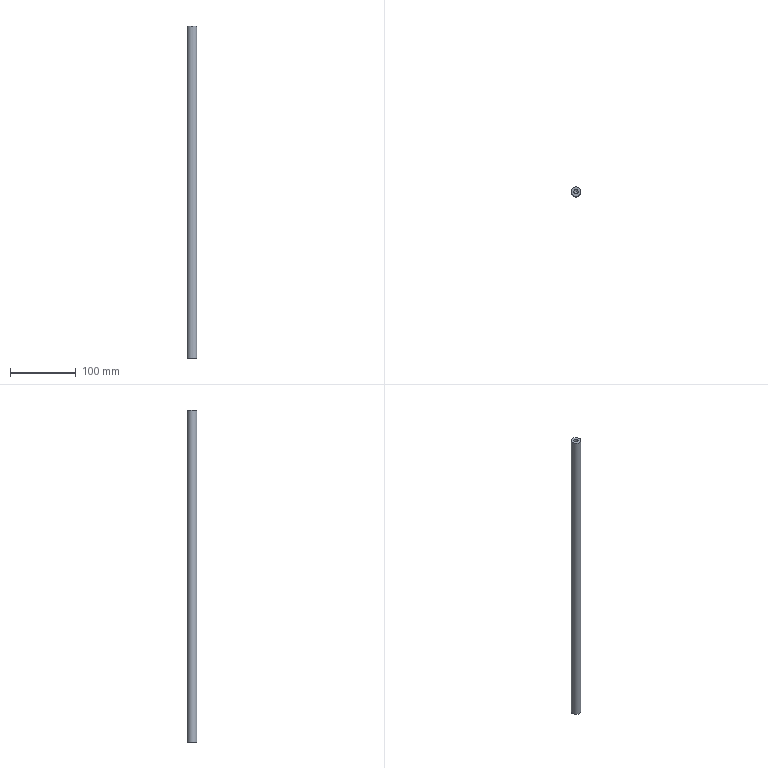Part | STEP file | axe506 | 1 solid | 7 faces | box 15 x 15 x 506 mm | volume 87993 mm3 | spline 4 | plane 2 | cylinder 1 | commonest cylinder face diameters 15 x1
STEP:
#1=CARTESIAN_POINT('',(0.,0.,0.));
#2=DIRECTION('',(0.,0.,1.));
#3=DIRECTION('',(1.,0.,0.));
#4=AXIS2_PLACEMENT_3D('',#1,#2,#3);
#5=CARTESIAN_POINT('',(3.324,0.,20.));
#6=VERTEX_POINT('',#5);
#7=CARTESIAN_POINT('',(-3.324,0.,20.));
#8=VERTEX_POINT('',#7);
#9=CARTESIAN_POINT('',(0.,0.,20.));
#10=DIRECTION('',(0.,0.,-1.));
#11=DIRECTION('',(-1.,0.,0.));
#12=AXIS2_PLACEMENT_3D('',#9,#10,#11);
#13=CIRCLE('',#12,3.324);
#14=CARTESIAN_POINT('',(3.324,0.,20.));
#15=CARTESIAN_POINT('',(3.324,-3.324,20.));
#16=CARTESIAN_POINT('',(0.,-3.324,20.));
#17=CARTESIAN_POINT('',(-3.324,-3.324,20.));
#18=CARTESIAN_POINT('',(-3.324,0.,20.));
#19=CARTESIAN_POINT('',(-3.324,3.324,20.));
#20=CARTESIAN_POINT('',(0.,3.324,20.));
#21=CARTESIAN_POINT('',(3.324,3.324,20.));
#22=CARTESIAN_POINT('',(3.324,0.,20.));
#23=CARTESIAN_POINT('',(0.,0.,21.997));
#24=CARTESIAN_POINT('',(0.,0.,21.997));
#25=CARTESIAN_POINT('',(0.,0.,21.997));
#26=CARTESIAN_POINT('',(0.,0.,21.997));
#27=CARTESIAN_POINT('',(0.,0.,21.997));
#28=CARTESIAN_POINT('',(0.,0.,21.997));
#29=CARTESIAN_POINT('',(0.,0.,21.997));
#30=CARTESIAN_POINT('',(0.,0.,21.997));
#31=CARTESIAN_POINT('',(0.,0.,21.997));
#32=(BOUNDED_SURFACE()B_SPLINE_SURFACE(1,2,((#14,#15,#16,#17,#18,#19,#20,#21,#22),(#23,#24,#25,#26,#27,#28,#29,#30,#31)),.UNSPECIFIED.,.F.,.T.,.F.)B_SPLINE_SURFACE_WITH_KNOTS((2,2),(1,2,2,2,2,2,1),(-1.167,1.167),(-2.61,0.,2.61,5.221,7.831,10.441,13.051),.UNSPECIFIED.)GEOMETRIC_REPRESENTATION_ITEM()RATIONAL_B_SPLINE_SURFACE(((1.,0.7071,1.,0.7071,1.,0.7071,1.,0.7071,1.),(1.,0.7071,1.,0.7071,1.,0.7071,1.,0.7071,1.)))REPRESENTATION_ITEM('')SURFACE());
#33=CARTESIAN_POINT('',(-1.167,-5.221));
#34=CARTESIAN_POINT('',(-1.167,-5.045));
#35=CARTESIAN_POINT('',(-1.167,-4.714));
#36=CARTESIAN_POINT('',(-1.167,-4.252));
#37=CARTESIAN_POINT('',(-1.167,-3.804));
#38=CARTESIAN_POINT('',(-1.167,-3.35));
#39=CARTESIAN_POINT('',(-1.167,-2.876));
#40=CARTESIAN_POINT('',(-1.167,-2.344));
#41=CARTESIAN_POINT('',(-1.167,-1.87));
#42=CARTESIAN_POINT('',(-1.167,-1.417));
#43=CARTESIAN_POINT('',(-1.167,-0.968));
#44=CARTESIAN_POINT('',(-1.167,-0.5094));
#45=CARTESIAN_POINT('',(-1.167,0.));
#46=CARTESIAN_POINT('',(-1.167,0.5094));
#47=CARTESIAN_POINT('',(-1.167,0.968));
#48=CARTESIAN_POINT('',(-1.167,1.417));
#49=CARTESIAN_POINT('',(-1.167,1.87));
#50=CARTESIAN_POINT('',(-1.167,2.344));
#51=CARTESIAN_POINT('',(-1.167,2.876));
#52=CARTESIAN_POINT('',(-1.167,3.35));
#53=CARTESIAN_POINT('',(-1.167,3.804));
#54=CARTESIAN_POINT('',(-1.167,4.252));
#55=CARTESIAN_POINT('',(-1.167,4.714));
#56=CARTESIAN_POINT('',(-1.167,5.045));
#57=CARTESIAN_POINT('',(-1.167,5.221));
#58=B_SPLINE_CURVE_WITH_KNOTS('',3,(#33,#34,#35,#36,#37,#38,#39,#40,#41,#42,#43,#44,#45,#46,#47,#48,#49,#50,#51,#52,#53,#54,#55,#56,#57),.UNSPECIFIED.,.F.,.F.,(4,1,1,1,1,1,1,1,1,1,1,1,1,1,1,1,1,1,1,1,1,1,4),(0.,0.2856,0.5712,0.8568,1.142,1.428,1.714,1.999,2.285,2.57,2.856,3.142,3.427,3.713,3.998,4.284,4.57,4.855,5.141,5.426,5.712,5.998,6.283),.QUASI_UNIFORM_KNOTS.);
#59=(GEOMETRIC_REPRESENTATION_CONTEXT(2)PARAMETRIC_REPRESENTATION_CONTEXT()REPRESENTATION_CONTEXT('',''));
#60=DEFINITIONAL_REPRESENTATION('',(#58),#59);
#61=PCURVE('',#32,#60);
#62=CARTESIAN_POINT('',(3.324,0.,0.));
#63=CARTESIAN_POINT('',(3.324,-3.324,0.));
#64=CARTESIAN_POINT('',(0.,-3.324,0.));
#65=CARTESIAN_POINT('',(-3.324,-3.324,0.));
#66=CARTESIAN_POINT('',(-3.324,0.,0.));
#67=CARTESIAN_POINT('',(-3.324,3.324,0.));
#68=CARTESIAN_POINT('',(0.,3.324,0.));
#69=CARTESIAN_POINT('',(3.324,3.324,0.));
#70=CARTESIAN_POINT('',(3.324,0.,0.));
#71=CARTESIAN_POINT('',(3.324,0.,20.));
#72=CARTESIAN_POINT('',(3.324,-3.324,20.));
#73=CARTESIAN_POINT('',(0.,-3.324,20.));
#74=CARTESIAN_POINT('',(-3.324,-3.324,20.));
#75=CARTESIAN_POINT('',(-3.324,0.,20.));
#76=CARTESIAN_POINT('',(-3.324,3.324,20.));
#77=CARTESIAN_POINT('',(0.,3.324,20.));
#78=CARTESIAN_POINT('',(3.324,3.324,20.));
#79=CARTESIAN_POINT('',(3.324,0.,20.));
#80=(BOUNDED_SURFACE()B_SPLINE_SURFACE(1,2,((#62,#63,#64,#65,#66,#67,#68,#69,#70),(#71,#72,#73,#74,#75,#76,#77,#78,#79)),.UNSPECIFIED.,.F.,.T.,.F.)B_SPLINE_SURFACE_WITH_KNOTS((2,2),(1,2,2,2,2,2,1),(-3.009,3.009),(-5.221,0.,5.221,10.441,15.662,20.882,26.103),.UNSPECIFIED.)GEOMETRIC_REPRESENTATION_ITEM()RATIONAL_B_SPLINE_SURFACE(((1.,0.7071,1.,0.7071,1.,0.7071,1.,0.7071,1.),(1.,0.7071,1.,0.7071,1.,0.7071,1.,0.7071,1.)))REPRESENTATION_ITEM('')SURFACE());
#81=CARTESIAN_POINT('',(3.009,20.882));
#82=CARTESIAN_POINT('',(3.009,21.058));
#83=CARTESIAN_POINT('',(3.009,21.399));
#84=CARTESIAN_POINT('',(3.009,21.887));
#85=CARTESIAN_POINT('',(3.009,22.357));
#86=CARTESIAN_POINT('',(3.009,22.816));
#87=CARTESIAN_POINT('',(3.009,23.268));
#88=CARTESIAN_POINT('',(3.009,23.717));
#89=CARTESIAN_POINT('',(3.009,24.169));
#90=CARTESIAN_POINT('',(3.009,24.627));
#91=CARTESIAN_POINT('',(3.009,25.098));
#92=CARTESIAN_POINT('',(3.009,25.585));
#93=CARTESIAN_POINT('',(3.009,26.103));
#94=CARTESIAN_POINT('',(3.009,26.621));
#95=CARTESIAN_POINT('',(3.009,27.107));
#96=CARTESIAN_POINT('',(3.009,27.578));
#97=CARTESIAN_POINT('',(3.009,28.037));
#98=CARTESIAN_POINT('',(3.009,28.488));
#99=CARTESIAN_POINT('',(3.009,28.938));
#100=CARTESIAN_POINT('',(3.009,29.389));
#101=CARTESIAN_POINT('',(3.009,29.848));
#102=CARTESIAN_POINT('',(3.009,30.319));
#103=CARTESIAN_POINT('',(3.009,30.806));
#104=CARTESIAN_POINT('',(3.009,31.148));
#105=CARTESIAN_POINT('',(3.009,31.323));
#106=B_SPLINE_CURVE_WITH_KNOTS('',3,(#81,#82,#83,#84,#85,#86,#87,#88,#89,#90,#91,#92,#93,#94,#95,#96,#97,#98,#99,#100,#101,#102,#103,#104,#105),.UNSPECIFIED.,.F.,.F.,(4,1,1,1,1,1,1,1,1,1,1,1,1,1,1,1,1,1,1,1,1,1,4),(3.142,3.284,3.427,3.57,3.713,3.856,3.998,4.141,4.284,4.427,4.57,4.712,4.855,4.998,5.141,5.284,5.426,5.569,5.712,5.855,5.998,6.14,6.283),.QUASI_UNIFORM_KNOTS.);
#107=(GEOMETRIC_REPRESENTATION_CONTEXT(2)PARAMETRIC_REPRESENTATION_CONTEXT()REPRESENTATION_CONTEXT('',''));
#108=DEFINITIONAL_REPRESENTATION('',(#106),#107);
#109=PCURVE('',#80,#108);
#110=SURFACE_CURVE('',#13,(#61,#109),.PCURVE_S1.);
#111=EDGE_CURVE('',#6,#8,#110,.T.);
#112=ORIENTED_EDGE('',*,*,#111,.F.);
#113=CARTESIAN_POINT('',(0.,0.,21.997));
#114=VERTEX_POINT('',#113);
#115=CARTESIAN_POINT('',(3.324,0.,20.));
#116=CARTESIAN_POINT('',(0.,0.,21.997));
#117=B_SPLINE_CURVE_WITH_KNOTS('',1,(#115,#116),.UNSPECIFIED.,.F.,.F.,(2,2),(-1.167,1.167),.PIECEWISE_BEZIER_KNOTS.);
#118=CARTESIAN_POINT('',(0.,0.));
#119=DIRECTION('',(1.,0.));
#120=VECTOR('',#119,1.);
#121=LINE('',#118,#120);
#122=(GEOMETRIC_REPRESENTATION_CONTEXT(2)PARAMETRIC_REPRESENTATION_CONTEXT()REPRESENTATION_CONTEXT('',''));
#123=DEFINITIONAL_REPRESENTATION('',(#121),#122);
#124=PCURVE('',#32,#123);
#125=CARTESIAN_POINT('',(0.,10.441));
#126=DIRECTION('',(1.,0.));
#127=VECTOR('',#126,1.);
#128=LINE('',#125,#127);
#129=(GEOMETRIC_REPRESENTATION_CONTEXT(2)PARAMETRIC_REPRESENTATION_CONTEXT()REPRESENTATION_CONTEXT('',''));
#130=DEFINITIONAL_REPRESENTATION('',(#128),#129);
#131=PCURVE('',#32,#130);
#132=SEAM_CURVE('',#117,(#124,#131),.PCURVE_S1.);
#133=EDGE_CURVE('',#6,#114,#132,.T.);
#134=ORIENTED_EDGE('',*,*,#133,.T.);
#135=ORIENTED_EDGE('',*,*,#133,.F.);
#136=CARTESIAN_POINT('',(0.,0.,20.));
#137=DIRECTION('',(0.,0.,-1.));
#138=DIRECTION('',(-1.,0.,0.));
#139=AXIS2_PLACEMENT_3D('',#136,#137,#138);
#140=CIRCLE('',#139,3.324);
#141=CARTESIAN_POINT('',(-1.167,5.221));
#142=CARTESIAN_POINT('',(-1.167,5.396));
#143=CARTESIAN_POINT('',(-1.167,5.727));
#144=CARTESIAN_POINT('',(-1.167,6.189));
#145=CARTESIAN_POINT('',(-1.167,6.637));
#146=CARTESIAN_POINT('',(-1.167,7.091));
#147=CARTESIAN_POINT('',(-1.167,7.565));
#148=CARTESIAN_POINT('',(-1.167,8.097));
#149=CARTESIAN_POINT('',(-1.167,8.571));
#150=CARTESIAN_POINT('',(-1.167,9.024));
#151=CARTESIAN_POINT('',(-1.167,9.473));
#152=CARTESIAN_POINT('',(-1.167,9.932));
#153=CARTESIAN_POINT('',(-1.167,10.441));
#154=CARTESIAN_POINT('',(-1.167,10.95));
#155=CARTESIAN_POINT('',(-1.167,11.409));
#156=CARTESIAN_POINT('',(-1.167,11.858));
#157=CARTESIAN_POINT('',(-1.167,12.311));
#158=CARTESIAN_POINT('',(-1.167,12.785));
#159=CARTESIAN_POINT('',(-1.167,13.318));
#160=CARTESIAN_POINT('',(-1.167,13.791));
#161=CARTESIAN_POINT('',(-1.167,14.245));
#162=CARTESIAN_POINT('',(-1.167,14.693));
#163=CARTESIAN_POINT('',(-1.167,15.155));
#164=CARTESIAN_POINT('',(-1.167,15.486));
#165=CARTESIAN_POINT('',(-1.167,15.662));
#166=B_SPLINE_CURVE_WITH_KNOTS('',3,(#141,#142,#143,#144,#145,#146,#147,#148,#149,#150,#151,#152,#153,#154,#155,#156,#157,#158,#159,#160,#161,#162,#163,#164,#165),.UNSPECIFIED.,.F.,.F.,(4,1,1,1,1,1,1,1,1,1,1,1,1,1,1,1,1,1,1,1,1,1,4),(0.,0.2856,0.5712,0.8568,1.142,1.428,1.714,1.999,2.285,2.57,2.856,3.142,3.427,3.713,3.998,4.284,4.57,4.855,5.141,5.426,5.712,5.998,6.283),.QUASI_UNIFORM_KNOTS.);
#167=(GEOMETRIC_REPRESENTATION_CONTEXT(2)PARAMETRIC_REPRESENTATION_CONTEXT()REPRESENTATION_CONTEXT('',''));
#168=DEFINITIONAL_REPRESENTATION('',(#166),#167);
#169=PCURVE('',#32,#168);
#170=CARTESIAN_POINT('',(3.009,10.441));
#171=CARTESIAN_POINT('',(3.009,10.617));
#172=CARTESIAN_POINT('',(3.009,10.958));
#173=CARTESIAN_POINT('',(3.009,11.446));
#174=CARTESIAN_POINT('',(3.009,11.916));
#175=CARTESIAN_POINT('',(3.009,12.375));
#176=CARTESIAN_POINT('',(3.009,12.827));
#177=CARTESIAN_POINT('',(3.009,13.276));
#178=CARTESIAN_POINT('',(3.009,13.728));
#179=CARTESIAN_POINT('',(3.009,14.186));
#180=CARTESIAN_POINT('',(3.009,14.657));
#181=CARTESIAN_POINT('',(3.009,15.143));
#182=CARTESIAN_POINT('',(3.009,15.662));
#183=CARTESIAN_POINT('',(3.009,16.18));
#184=CARTESIAN_POINT('',(3.009,16.666));
#185=CARTESIAN_POINT('',(3.009,17.137));
#186=CARTESIAN_POINT('',(3.009,17.596));
#187=CARTESIAN_POINT('',(3.009,18.047));
#188=CARTESIAN_POINT('',(3.009,18.497));
#189=CARTESIAN_POINT('',(3.009,18.948));
#190=CARTESIAN_POINT('',(3.009,19.407));
#191=CARTESIAN_POINT('',(3.009,19.877));
#192=CARTESIAN_POINT('',(3.009,20.365));
#193=CARTESIAN_POINT('',(3.009,20.707));
#194=CARTESIAN_POINT('',(3.009,20.882));
#195=B_SPLINE_CURVE_WITH_KNOTS('',3,(#170,#171,#172,#173,#174,#175,#176,#177,#178,#179,#180,#181,#182,#183,#184,#185,#186,#187,#188,#189,#190,#191,#192,#193,#194),.UNSPECIFIED.,.F.,.F.,(4,1,1,1,1,1,1,1,1,1,1,1,1,1,1,1,1,1,1,1,1,1,4),(0.,0.1428,0.2856,0.4284,0.5712,0.714,0.8568,0.9996,1.142,1.285,1.428,1.571,1.714,1.856,1.999,2.142,2.285,2.428,2.57,2.713,2.856,2.999,3.142),.QUASI_UNIFORM_KNOTS.);
#196=(GEOMETRIC_REPRESENTATION_CONTEXT(2)PARAMETRIC_REPRESENTATION_CONTEXT()REPRESENTATION_CONTEXT('',''));
#197=DEFINITIONAL_REPRESENTATION('',(#195),#196);
#198=PCURVE('',#80,#197);
#199=SURFACE_CURVE('',#140,(#169,#198),.PCURVE_S1.);
#200=EDGE_CURVE('',#8,#6,#199,.T.);
#201=ORIENTED_EDGE('',*,*,#200,.F.);
#202=EDGE_LOOP('',(#112,#134,#135,#201));
#203=FACE_BOUND('',#202,.F.);
#204=ADVANCED_FACE('',(#203),#32,.F.);
#205=CARTESIAN_POINT('',(-3.324,0.,0.));
#206=VERTEX_POINT('',#205);
#207=CARTESIAN_POINT('',(0.,0.,0.));
#208=DIRECTION('',(0.,0.,1.));
#209=DIRECTION('',(-1.,0.,0.));
#210=AXIS2_PLACEMENT_3D('',#207,#208,#209);
#211=CIRCLE('',#210,3.324);
#212=CARTESIAN_POINT('',(-3.009,31.323));
#213=CARTESIAN_POINT('',(-3.009,30.973));
#214=CARTESIAN_POINT('',(-3.009,30.31));
#215=CARTESIAN_POINT('',(-3.009,29.386));
#216=CARTESIAN_POINT('',(-3.009,28.49));
#217=CARTESIAN_POINT('',(-3.009,27.583));
#218=CARTESIAN_POINT('',(-3.009,26.635));
#219=CARTESIAN_POINT('',(-3.009,25.57));
#220=CARTESIAN_POINT('',(-3.009,24.622));
#221=CARTESIAN_POINT('',(-3.009,23.716));
#222=CARTESIAN_POINT('',(-3.009,22.818));
#223=CARTESIAN_POINT('',(-3.009,21.901));
#224=CARTESIAN_POINT('',(-3.009,20.882));
#225=CARTESIAN_POINT('',(-3.009,19.863));
#226=CARTESIAN_POINT('',(-3.009,18.946));
#227=CARTESIAN_POINT('',(-3.009,18.048));
#228=CARTESIAN_POINT('',(-3.009,17.142));
#229=CARTESIAN_POINT('',(-3.009,16.194));
#230=CARTESIAN_POINT('',(-3.009,15.129));
#231=CARTESIAN_POINT('',(-3.009,14.181));
#232=CARTESIAN_POINT('',(-3.009,13.275));
#233=CARTESIAN_POINT('',(-3.009,12.378));
#234=CARTESIAN_POINT('',(-3.009,11.455));
#235=CARTESIAN_POINT('',(-3.009,10.792));
#236=CARTESIAN_POINT('',(-3.009,10.441));
#237=B_SPLINE_CURVE_WITH_KNOTS('',3,(#212,#213,#214,#215,#216,#217,#218,#219,#220,#221,#222,#223,#224,#225,#226,#227,#228,#229,#230,#231,#232,#233,#234,#235,#236),.UNSPECIFIED.,.F.,.F.,(4,1,1,1,1,1,1,1,1,1,1,1,1,1,1,1,1,1,1,1,1,1,4),(0.,0.2856,0.5712,0.8568,1.142,1.428,1.714,1.999,2.285,2.57,2.856,3.142,3.427,3.713,3.998,4.284,4.57,4.855,5.141,5.426,5.712,5.998,6.283),.QUASI_UNIFORM_KNOTS.);
#238=(GEOMETRIC_REPRESENTATION_CONTEXT(2)PARAMETRIC_REPRESENTATION_CONTEXT()REPRESENTATION_CONTEXT('',''));
#239=DEFINITIONAL_REPRESENTATION('',(#237),#238);
#240=PCURVE('',#80,#239);
#241=CARTESIAN_POINT('',(0.,0.,0.));
#242=DIRECTION('',(0.,0.,-1.));
#243=DIRECTION('',(-1.,0.,0.));
#244=AXIS2_PLACEMENT_3D('',#241,#242,#243);
#245=PLANE('',#244);
#246=CARTESIAN_POINT('',(3.324,0.));
#247=CARTESIAN_POINT('',(3.324,-5.756));
#248=CARTESIAN_POINT('',(-1.662,-2.878));
#249=CARTESIAN_POINT('',(-6.647,0.));
#250=CARTESIAN_POINT('',(-1.662,2.878));
#251=CARTESIAN_POINT('',(3.324,5.756));
#252=CARTESIAN_POINT('',(3.324,0.));
#253=(BOUNDED_CURVE()B_SPLINE_CURVE(2,(#246,#247,#248,#249,#250,#251,#252),.UNSPECIFIED.,.T.,.F.)B_SPLINE_CURVE_WITH_KNOTS((1,2,2,2,2,1),(-2.094,0.,2.094,4.189,6.283,8.378),.UNSPECIFIED.)CURVE()GEOMETRIC_REPRESENTATION_ITEM()RATIONAL_B_SPLINE_CURVE((1.,0.5,1.,0.5,1.,0.5,1.))REPRESENTATION_ITEM(''));
#254=(GEOMETRIC_REPRESENTATION_CONTEXT(2)PARAMETRIC_REPRESENTATION_CONTEXT()REPRESENTATION_CONTEXT('',''));
#255=DEFINITIONAL_REPRESENTATION('',(#253),#254);
#256=PCURVE('',#245,#255);
#257=SURFACE_CURVE('',#211,(#240,#256),.PCURVE_S1.);
#258=EDGE_CURVE('',#206,#206,#257,.T.);
#259=ORIENTED_EDGE('',*,*,#258,.T.);
#260=CARTESIAN_POINT('',(-3.324,0.,0.));
#261=CARTESIAN_POINT('',(-3.324,0.,20.));
#262=B_SPLINE_CURVE_WITH_KNOTS('',1,(#260,#261),.UNSPECIFIED.,.F.,.F.,(2,2),(-3.009,3.009),.PIECEWISE_BEZIER_KNOTS.);
#263=CARTESIAN_POINT('',(0.,10.441));
#264=DIRECTION('',(1.,0.));
#265=VECTOR('',#264,1.);
#266=LINE('',#263,#265);
#267=(GEOMETRIC_REPRESENTATION_CONTEXT(2)PARAMETRIC_REPRESENTATION_CONTEXT()REPRESENTATION_CONTEXT('',''));
#268=DEFINITIONAL_REPRESENTATION('',(#266),#267);
#269=PCURVE('',#80,#268);
#270=CARTESIAN_POINT('',(0.,31.323));
#271=DIRECTION('',(1.,0.));
#272=VECTOR('',#271,1.);
#273=LINE('',#270,#272);
#274=(GEOMETRIC_REPRESENTATION_CONTEXT(2)PARAMETRIC_REPRESENTATION_CONTEXT()REPRESENTATION_CONTEXT('',''));
#275=DEFINITIONAL_REPRESENTATION('',(#273),#274);
#276=PCURVE('',#80,#275);
#277=SEAM_CURVE('',#262,(#269,#276),.PCURVE_S1.);
#278=EDGE_CURVE('',#206,#8,#277,.T.);
#279=ORIENTED_EDGE('',*,*,#278,.T.);
#280=ORIENTED_EDGE('',*,*,#200,.T.);
#281=ORIENTED_EDGE('',*,*,#111,.T.);
#282=ORIENTED_EDGE('',*,*,#278,.F.);
#283=EDGE_LOOP('',(#259,#279,#280,#281,#282));
#284=FACE_BOUND('',#283,.F.);
#285=ADVANCED_FACE('',(#284),#80,.F.);
#286=CARTESIAN_POINT('',(-3.324,0.,486.));
#287=VERTEX_POINT('',#286);
#288=CARTESIAN_POINT('',(3.324,0.,486.));
#289=VERTEX_POINT('',#288);
#290=CARTESIAN_POINT('',(0.,0.,486.));
#291=DIRECTION('',(0.,0.,1.));
#292=DIRECTION('',(1.,0.,0.));
#293=AXIS2_PLACEMENT_3D('',#290,#291,#292);
#294=CIRCLE('',#293,3.324);
#295=CARTESIAN_POINT('',(-3.324,0.,486.));
#296=CARTESIAN_POINT('',(-3.324,-3.324,486.));
#297=CARTESIAN_POINT('',(0.,-3.324,486.));
#298=CARTESIAN_POINT('',(3.324,-3.324,486.));
#299=CARTESIAN_POINT('',(3.324,0.,486.));
#300=CARTESIAN_POINT('',(3.324,3.324,486.));
#301=CARTESIAN_POINT('',(0.,3.324,486.));
#302=CARTESIAN_POINT('',(-3.324,3.324,486.));
#303=CARTESIAN_POINT('',(-3.324,0.,486.));
#304=CARTESIAN_POINT('',(0.,0.,484.003));
#305=CARTESIAN_POINT('',(0.,0.,484.003));
#306=CARTESIAN_POINT('',(0.,0.,484.003));
#307=CARTESIAN_POINT('',(0.,0.,484.003));
#308=CARTESIAN_POINT('',(0.,0.,484.003));
#309=CARTESIAN_POINT('',(0.,0.,484.003));
#310=CARTESIAN_POINT('',(0.,0.,484.003));
#311=CARTESIAN_POINT('',(0.,0.,484.003));
#312=CARTESIAN_POINT('',(0.,0.,484.003));
#313=(BOUNDED_SURFACE()B_SPLINE_SURFACE(1,2,((#295,#296,#297,#298,#299,#300,#301,#302,#303),(#304,#305,#306,#307,#308,#309,#310,#311,#312)),.UNSPECIFIED.,.F.,.T.,.F.)B_SPLINE_SURFACE_WITH_KNOTS((2,2),(1,2,2,2,2,2,1),(-1.167,1.167),(-2.61,0.,2.61,5.221,7.831,10.441,13.051),.UNSPECIFIED.)GEOMETRIC_REPRESENTATION_ITEM()RATIONAL_B_SPLINE_SURFACE(((1.,0.7071,1.,0.7071,1.,0.7071,1.,0.7071,1.),(1.,0.7071,1.,0.7071,1.,0.7071,1.,0.7071,1.)))REPRESENTATION_ITEM('')SURFACE());
#314=CARTESIAN_POINT('',(-1.167,-5.221));
#315=CARTESIAN_POINT('',(-1.167,-5.045));
#316=CARTESIAN_POINT('',(-1.167,-4.714));
#317=CARTESIAN_POINT('',(-1.167,-4.252));
#318=CARTESIAN_POINT('',(-1.167,-3.804));
#319=CARTESIAN_POINT('',(-1.167,-3.35));
#320=CARTESIAN_POINT('',(-1.167,-2.876));
#321=CARTESIAN_POINT('',(-1.167,-2.344));
#322=CARTESIAN_POINT('',(-1.167,-1.87));
#323=CARTESIAN_POINT('',(-1.167,-1.417));
#324=CARTESIAN_POINT('',(-1.167,-0.968));
#325=CARTESIAN_POINT('',(-1.167,-0.5094));
#326=CARTESIAN_POINT('',(-1.167,0.));
#327=CARTESIAN_POINT('',(-1.167,0.5094));
#328=CARTESIAN_POINT('',(-1.167,0.968));
#329=CARTESIAN_POINT('',(-1.167,1.417));
#330=CARTESIAN_POINT('',(-1.167,1.87));
#331=CARTESIAN_POINT('',(-1.167,2.344));
#332=CARTESIAN_POINT('',(-1.167,2.876));
#333=CARTESIAN_POINT('',(-1.167,3.35));
#334=CARTESIAN_POINT('',(-1.167,3.804));
#335=CARTESIAN_POINT('',(-1.167,4.252));
#336=CARTESIAN_POINT('',(-1.167,4.714));
#337=CARTESIAN_POINT('',(-1.167,5.045));
#338=CARTESIAN_POINT('',(-1.167,5.221));
#339=B_SPLINE_CURVE_WITH_KNOTS('',3,(#314,#315,#316,#317,#318,#319,#320,#321,#322,#323,#324,#325,#326,#327,#328,#329,#330,#331,#332,#333,#334,#335,#336,#337,#338),.UNSPECIFIED.,.F.,.F.,(4,1,1,1,1,1,1,1,1,1,1,1,1,1,1,1,1,1,1,1,1,1,4),(0.,0.2856,0.5712,0.8568,1.142,1.428,1.714,1.999,2.285,2.57,2.856,3.142,3.427,3.713,3.998,4.284,4.57,4.855,5.141,5.426,5.712,5.998,6.283),.QUASI_UNIFORM_KNOTS.);
#340=(GEOMETRIC_REPRESENTATION_CONTEXT(2)PARAMETRIC_REPRESENTATION_CONTEXT()REPRESENTATION_CONTEXT('',''));
#341=DEFINITIONAL_REPRESENTATION('',(#339),#340);
#342=PCURVE('',#313,#341);
#343=CARTESIAN_POINT('',(-3.324,0.,506.));
#344=CARTESIAN_POINT('',(-3.324,-3.324,506.));
#345=CARTESIAN_POINT('',(0.,-3.324,506.));
#346=CARTESIAN_POINT('',(3.324,-3.324,506.));
#347=CARTESIAN_POINT('',(3.324,0.,506.));
#348=CARTESIAN_POINT('',(3.324,3.324,506.));
#349=CARTESIAN_POINT('',(0.,3.324,506.));
#350=CARTESIAN_POINT('',(-3.324,3.324,506.));
#351=CARTESIAN_POINT('',(-3.324,0.,506.));
#352=CARTESIAN_POINT('',(-3.324,0.,486.));
#353=CARTESIAN_POINT('',(-3.324,-3.324,486.));
#354=CARTESIAN_POINT('',(0.,-3.324,486.));
#355=CARTESIAN_POINT('',(3.324,-3.324,486.));
#356=CARTESIAN_POINT('',(3.324,0.,486.));
#357=CARTESIAN_POINT('',(3.324,3.324,486.));
#358=CARTESIAN_POINT('',(0.,3.324,486.));
#359=CARTESIAN_POINT('',(-3.324,3.324,486.));
#360=CARTESIAN_POINT('',(-3.324,0.,486.));
#361=(BOUNDED_SURFACE()B_SPLINE_SURFACE(1,2,((#343,#344,#345,#346,#347,#348,#349,#350,#351),(#352,#353,#354,#355,#356,#357,#358,#359,#360)),.UNSPECIFIED.,.F.,.T.,.F.)B_SPLINE_SURFACE_WITH_KNOTS((2,2),(1,2,2,2,2,2,1),(-3.009,3.009),(-5.221,0.,5.221,10.441,15.662,20.882,26.103),.UNSPECIFIED.)GEOMETRIC_REPRESENTATION_ITEM()RATIONAL_B_SPLINE_SURFACE(((1.,0.7071,1.,0.7071,1.,0.7071,1.,0.7071,1.),(1.,0.7071,1.,0.7071,1.,0.7071,1.,0.7071,1.)))REPRESENTATION_ITEM('')SURFACE());
#362=CARTESIAN_POINT('',(3.009,20.882));
#363=CARTESIAN_POINT('',(3.009,21.058));
#364=CARTESIAN_POINT('',(3.009,21.399));
#365=CARTESIAN_POINT('',(3.009,21.887));
#366=CARTESIAN_POINT('',(3.009,22.357));
#367=CARTESIAN_POINT('',(3.009,22.816));
#368=CARTESIAN_POINT('',(3.009,23.268));
#369=CARTESIAN_POINT('',(3.009,23.717));
#370=CARTESIAN_POINT('',(3.009,24.169));
#371=CARTESIAN_POINT('',(3.009,24.627));
#372=CARTESIAN_POINT('',(3.009,25.098));
#373=CARTESIAN_POINT('',(3.009,25.585));
#374=CARTESIAN_POINT('',(3.009,26.103));
#375=CARTESIAN_POINT('',(3.009,26.621));
#376=CARTESIAN_POINT('',(3.009,27.107));
#377=CARTESIAN_POINT('',(3.009,27.578));
#378=CARTESIAN_POINT('',(3.009,28.037));
#379=CARTESIAN_POINT('',(3.009,28.488));
#380=CARTESIAN_POINT('',(3.009,28.938));
#381=CARTESIAN_POINT('',(3.009,29.389));
#382=CARTESIAN_POINT('',(3.009,29.848));
#383=CARTESIAN_POINT('',(3.009,30.319));
#384=CARTESIAN_POINT('',(3.009,30.806));
#385=CARTESIAN_POINT('',(3.009,31.148));
#386=CARTESIAN_POINT('',(3.009,31.323));
#387=B_SPLINE_CURVE_WITH_KNOTS('',3,(#362,#363,#364,#365,#366,#367,#368,#369,#370,#371,#372,#373,#374,#375,#376,#377,#378,#379,#380,#381,#382,#383,#384,#385,#386),.UNSPECIFIED.,.F.,.F.,(4,1,1,1,1,1,1,1,1,1,1,1,1,1,1,1,1,1,1,1,1,1,4),(3.142,3.284,3.427,3.57,3.713,3.856,3.998,4.141,4.284,4.427,4.57,4.712,4.855,4.998,5.141,5.284,5.426,5.569,5.712,5.855,5.998,6.14,6.283),.QUASI_UNIFORM_KNOTS.);
#388=(GEOMETRIC_REPRESENTATION_CONTEXT(2)PARAMETRIC_REPRESENTATION_CONTEXT()REPRESENTATION_CONTEXT('',''));
#389=DEFINITIONAL_REPRESENTATION('',(#387),#388);
#390=PCURVE('',#361,#389);
#391=SURFACE_CURVE('',#294,(#342,#390),.PCURVE_S1.);
#392=EDGE_CURVE('',#287,#289,#391,.T.);
#393=ORIENTED_EDGE('',*,*,#392,.F.);
#394=CARTESIAN_POINT('',(0.,0.,484.003));
#395=VERTEX_POINT('',#394);
#396=CARTESIAN_POINT('',(-3.324,0.,486.));
#397=CARTESIAN_POINT('',(0.,0.,484.003));
#398=B_SPLINE_CURVE_WITH_KNOTS('',1,(#396,#397),.UNSPECIFIED.,.F.,.F.,(2,2),(-1.167,1.167),.PIECEWISE_BEZIER_KNOTS.);
#399=CARTESIAN_POINT('',(0.,0.));
#400=DIRECTION('',(1.,0.));
#401=VECTOR('',#400,1.);
#402=LINE('',#399,#401);
#403=(GEOMETRIC_REPRESENTATION_CONTEXT(2)PARAMETRIC_REPRESENTATION_CONTEXT()REPRESENTATION_CONTEXT('',''));
#404=DEFINITIONAL_REPRESENTATION('',(#402),#403);
#405=PCURVE('',#313,#404);
#406=CARTESIAN_POINT('',(0.,10.441));
#407=DIRECTION('',(1.,0.));
#408=VECTOR('',#407,1.);
#409=LINE('',#406,#408);
#410=(GEOMETRIC_REPRESENTATION_CONTEXT(2)PARAMETRIC_REPRESENTATION_CONTEXT()REPRESENTATION_CONTEXT('',''));
#411=DEFINITIONAL_REPRESENTATION('',(#409),#410);
#412=PCURVE('',#313,#411);
#413=SEAM_CURVE('',#398,(#405,#412),.PCURVE_S1.);
#414=EDGE_CURVE('',#287,#395,#413,.T.);
#415=ORIENTED_EDGE('',*,*,#414,.T.);
#416=ORIENTED_EDGE('',*,*,#414,.F.);
#417=CARTESIAN_POINT('',(0.,0.,486.));
#418=DIRECTION('',(0.,0.,1.));
#419=DIRECTION('',(1.,0.,0.));
#420=AXIS2_PLACEMENT_3D('',#417,#418,#419);
#421=CIRCLE('',#420,3.324);
#422=CARTESIAN_POINT('',(-1.167,5.221));
#423=CARTESIAN_POINT('',(-1.167,5.396));
#424=CARTESIAN_POINT('',(-1.167,5.727));
#425=CARTESIAN_POINT('',(-1.167,6.189));
#426=CARTESIAN_POINT('',(-1.167,6.637));
#427=CARTESIAN_POINT('',(-1.167,7.091));
#428=CARTESIAN_POINT('',(-1.167,7.565));
#429=CARTESIAN_POINT('',(-1.167,8.097));
#430=CARTESIAN_POINT('',(-1.167,8.571));
#431=CARTESIAN_POINT('',(-1.167,9.024));
#432=CARTESIAN_POINT('',(-1.167,9.473));
#433=CARTESIAN_POINT('',(-1.167,9.932));
#434=CARTESIAN_POINT('',(-1.167,10.441));
#435=CARTESIAN_POINT('',(-1.167,10.95));
#436=CARTESIAN_POINT('',(-1.167,11.409));
#437=CARTESIAN_POINT('',(-1.167,11.858));
#438=CARTESIAN_POINT('',(-1.167,12.311));
#439=CARTESIAN_POINT('',(-1.167,12.785));
#440=CARTESIAN_POINT('',(-1.167,13.318));
#441=CARTESIAN_POINT('',(-1.167,13.791));
#442=CARTESIAN_POINT('',(-1.167,14.245));
#443=CARTESIAN_POINT('',(-1.167,14.693));
#444=CARTESIAN_POINT('',(-1.167,15.155));
#445=CARTESIAN_POINT('',(-1.167,15.486));
#446=CARTESIAN_POINT('',(-1.167,15.662));
#447=B_SPLINE_CURVE_WITH_KNOTS('',3,(#422,#423,#424,#425,#426,#427,#428,#429,#430,#431,#432,#433,#434,#435,#436,#437,#438,#439,#440,#441,#442,#443,#444,#445,#446),.UNSPECIFIED.,.F.,.F.,(4,1,1,1,1,1,1,1,1,1,1,1,1,1,1,1,1,1,1,1,1,1,4),(0.,0.2856,0.5712,0.8568,1.142,1.428,1.714,1.999,2.285,2.57,2.856,3.142,3.427,3.713,3.998,4.284,4.57,4.855,5.141,5.426,5.712,5.998,6.283),.QUASI_UNIFORM_KNOTS.);
#448=(GEOMETRIC_REPRESENTATION_CONTEXT(2)PARAMETRIC_REPRESENTATION_CONTEXT()REPRESENTATION_CONTEXT('',''));
#449=DEFINITIONAL_REPRESENTATION('',(#447),#448);
#450=PCURVE('',#313,#449);
#451=CARTESIAN_POINT('',(3.009,10.441));
#452=CARTESIAN_POINT('',(3.009,10.617));
#453=CARTESIAN_POINT('',(3.009,10.958));
#454=CARTESIAN_POINT('',(3.009,11.446));
#455=CARTESIAN_POINT('',(3.009,11.916));
#456=CARTESIAN_POINT('',(3.009,12.375));
#457=CARTESIAN_POINT('',(3.009,12.827));
#458=CARTESIAN_POINT('',(3.009,13.276));
#459=CARTESIAN_POINT('',(3.009,13.728));
#460=CARTESIAN_POINT('',(3.009,14.186));
#461=CARTESIAN_POINT('',(3.009,14.657));
#462=CARTESIAN_POINT('',(3.009,15.143));
#463=CARTESIAN_POINT('',(3.009,15.662));
#464=CARTESIAN_POINT('',(3.009,16.18));
#465=CARTESIAN_POINT('',(3.009,16.666));
#466=CARTESIAN_POINT('',(3.009,17.137));
#467=CARTESIAN_POINT('',(3.009,17.596));
#468=CARTESIAN_POINT('',(3.009,18.047));
#469=CARTESIAN_POINT('',(3.009,18.497));
#470=CARTESIAN_POINT('',(3.009,18.948));
#471=CARTESIAN_POINT('',(3.009,19.407));
#472=CARTESIAN_POINT('',(3.009,19.877));
#473=CARTESIAN_POINT('',(3.009,20.365));
#474=CARTESIAN_POINT('',(3.009,20.707));
#475=CARTESIAN_POINT('',(3.009,20.882));
#476=B_SPLINE_CURVE_WITH_KNOTS('',3,(#451,#452,#453,#454,#455,#456,#457,#458,#459,#460,#461,#462,#463,#464,#465,#466,#467,#468,#469,#470,#471,#472,#473,#474,#475),.UNSPECIFIED.,.F.,.F.,(4,1,1,1,1,1,1,1,1,1,1,1,1,1,1,1,1,1,1,1,1,1,4),(0.,0.1428,0.2856,0.4284,0.5712,0.714,0.8568,0.9996,1.142,1.285,1.428,1.571,1.714,1.856,1.999,2.142,2.285,2.428,2.57,2.713,2.856,2.999,3.142),.QUASI_UNIFORM_KNOTS.);
#477=(GEOMETRIC_REPRESENTATION_CONTEXT(2)PARAMETRIC_REPRESENTATION_CONTEXT()REPRESENTATION_CONTEXT('',''));
#478=DEFINITIONAL_REPRESENTATION('',(#476),#477);
#479=PCURVE('',#361,#478);
#480=SURFACE_CURVE('',#421,(#450,#479),.PCURVE_S1.);
#481=EDGE_CURVE('',#289,#287,#480,.T.);
#482=ORIENTED_EDGE('',*,*,#481,.F.);
#483=EDGE_LOOP('',(#393,#415,#416,#482));
#484=FACE_BOUND('',#483,.F.);
#485=ADVANCED_FACE('',(#484),#313,.F.);
#486=CARTESIAN_POINT('',(3.324,0.,506.));
#487=VERTEX_POINT('',#486);
#488=CARTESIAN_POINT('',(0.,0.,506.));
#489=DIRECTION('',(0.,0.,-1.));
#490=DIRECTION('',(1.,0.,0.));
#491=AXIS2_PLACEMENT_3D('',#488,#489,#490);
#492=CIRCLE('',#491,3.324);
#493=CARTESIAN_POINT('',(-3.009,31.323));
#494=CARTESIAN_POINT('',(-3.009,30.973));
#495=CARTESIAN_POINT('',(-3.009,30.31));
#496=CARTESIAN_POINT('',(-3.009,29.386));
#497=CARTESIAN_POINT('',(-3.009,28.49));
#498=CARTESIAN_POINT('',(-3.009,27.583));
#499=CARTESIAN_POINT('',(-3.009,26.635));
#500=CARTESIAN_POINT('',(-3.009,25.57));
#501=CARTESIAN_POINT('',(-3.009,24.622));
#502=CARTESIAN_POINT('',(-3.009,23.716));
#503=CARTESIAN_POINT('',(-3.009,22.818));
#504=CARTESIAN_POINT('',(-3.009,21.901));
#505=CARTESIAN_POINT('',(-3.009,20.882));
#506=CARTESIAN_POINT('',(-3.009,19.863));
#507=CARTESIAN_POINT('',(-3.009,18.946));
#508=CARTESIAN_POINT('',(-3.009,18.048));
#509=CARTESIAN_POINT('',(-3.009,17.142));
#510=CARTESIAN_POINT('',(-3.009,16.194));
#511=CARTESIAN_POINT('',(-3.009,15.129));
#512=CARTESIAN_POINT('',(-3.009,14.181));
#513=CARTESIAN_POINT('',(-3.009,13.275));
#514=CARTESIAN_POINT('',(-3.009,12.378));
#515=CARTESIAN_POINT('',(-3.009,11.455));
#516=CARTESIAN_POINT('',(-3.009,10.792));
#517=CARTESIAN_POINT('',(-3.009,10.441));
#518=B_SPLINE_CURVE_WITH_KNOTS('',3,(#493,#494,#495,#496,#497,#498,#499,#500,#501,#502,#503,#504,#505,#506,#507,#508,#509,#510,#511,#512,#513,#514,#515,#516,#517),.UNSPECIFIED.,.F.,.F.,(4,1,1,1,1,1,1,1,1,1,1,1,1,1,1,1,1,1,1,1,1,1,4),(0.,0.2856,0.5712,0.8568,1.142,1.428,1.714,1.999,2.285,2.57,2.856,3.142,3.427,3.713,3.998,4.284,4.57,4.855,5.141,5.426,5.712,5.998,6.283),.QUASI_UNIFORM_KNOTS.);
#519=(GEOMETRIC_REPRESENTATION_CONTEXT(2)PARAMETRIC_REPRESENTATION_CONTEXT()REPRESENTATION_CONTEXT('',''));
#520=DEFINITIONAL_REPRESENTATION('',(#518),#519);
#521=PCURVE('',#361,#520);
#522=CARTESIAN_POINT('',(0.,0.,506.));
#523=DIRECTION('',(0.,0.,-1.));
#524=DIRECTION('',(-1.,0.,0.));
#525=AXIS2_PLACEMENT_3D('',#522,#523,#524);
#526=PLANE('',#525);
#527=CARTESIAN_POINT('',(0.,0.));
#528=DIRECTION('',(-1.,0.));
#529=AXIS2_PLACEMENT_2D('',#527,#528);
#530=CIRCLE('',#529,3.324);
#531=(GEOMETRIC_REPRESENTATION_CONTEXT(2)PARAMETRIC_REPRESENTATION_CONTEXT()REPRESENTATION_CONTEXT('',''));
#532=DEFINITIONAL_REPRESENTATION('',(#530),#531);
#533=PCURVE('',#526,#532);
#534=SURFACE_CURVE('',#492,(#521,#533),.PCURVE_S1.);
#535=EDGE_CURVE('',#487,#487,#534,.T.);
#536=ORIENTED_EDGE('',*,*,#535,.T.);
#537=CARTESIAN_POINT('',(3.324,0.,506.));
#538=CARTESIAN_POINT('',(3.324,0.,486.));
#539=B_SPLINE_CURVE_WITH_KNOTS('',1,(#537,#538),.UNSPECIFIED.,.F.,.F.,(2,2),(-3.009,3.009),.PIECEWISE_BEZIER_KNOTS.);
#540=CARTESIAN_POINT('',(0.,10.441));
#541=DIRECTION('',(1.,0.));
#542=VECTOR('',#541,1.);
#543=LINE('',#540,#542);
#544=(GEOMETRIC_REPRESENTATION_CONTEXT(2)PARAMETRIC_REPRESENTATION_CONTEXT()REPRESENTATION_CONTEXT('',''));
#545=DEFINITIONAL_REPRESENTATION('',(#543),#544);
#546=PCURVE('',#361,#545);
#547=CARTESIAN_POINT('',(0.,31.323));
#548=DIRECTION('',(1.,0.));
#549=VECTOR('',#548,1.);
#550=LINE('',#547,#549);
#551=(GEOMETRIC_REPRESENTATION_CONTEXT(2)PARAMETRIC_REPRESENTATION_CONTEXT()REPRESENTATION_CONTEXT('',''));
#552=DEFINITIONAL_REPRESENTATION('',(#550),#551);
#553=PCURVE('',#361,#552);
#554=SEAM_CURVE('',#539,(#546,#553),.PCURVE_S1.);
#555=EDGE_CURVE('',#487,#289,#554,.T.);
#556=ORIENTED_EDGE('',*,*,#555,.T.);
#557=ORIENTED_EDGE('',*,*,#481,.T.);
#558=ORIENTED_EDGE('',*,*,#392,.T.);
#559=ORIENTED_EDGE('',*,*,#555,.F.);
#560=EDGE_LOOP('',(#536,#556,#557,#558,#559));
#561=FACE_BOUND('',#560,.F.);
#562=ADVANCED_FACE('',(#561),#361,.F.);
#563=CARTESIAN_POINT('',(7.5,0.,506.));
#564=VERTEX_POINT('',#563);
#565=CARTESIAN_POINT('',(0.,0.,506.));
#566=DIRECTION('',(0.,0.,-1.));
#567=DIRECTION('',(-1.,0.,0.));
#568=AXIS2_PLACEMENT_3D('',#565,#566,#567);
#569=CIRCLE('',#568,7.5);
#570=CARTESIAN_POINT('',(0.,0.,0.));
#571=DIRECTION('',(0.,0.,1.));
#572=DIRECTION('',(-1.,0.,0.));
#573=AXIS2_PLACEMENT_3D('',#570,#571,#572);
#574=CYLINDRICAL_SURFACE('',#573,7.5);
#575=CARTESIAN_POINT('',(12.566,506.));
#576=DIRECTION('',(-1.,0.));
#577=VECTOR('',#576,1.);
#578=LINE('',#575,#577);
#579=(GEOMETRIC_REPRESENTATION_CONTEXT(2)PARAMETRIC_REPRESENTATION_CONTEXT()REPRESENTATION_CONTEXT('',''));
#580=DEFINITIONAL_REPRESENTATION('',(#578),#579);
#581=PCURVE('',#574,#580);
#582=CARTESIAN_POINT('',(0.,0.));
#583=DIRECTION('',(1.,0.));
#584=AXIS2_PLACEMENT_2D('',#582,#583);
#585=CIRCLE('',#584,7.5);
#586=(GEOMETRIC_REPRESENTATION_CONTEXT(2)PARAMETRIC_REPRESENTATION_CONTEXT()REPRESENTATION_CONTEXT('',''));
#587=DEFINITIONAL_REPRESENTATION('',(#585),#586);
#588=PCURVE('',#526,#587);
#589=SURFACE_CURVE('',#569,(#581,#588),.PCURVE_S1.);
#590=EDGE_CURVE('',#564,#564,#589,.T.);
#591=ORIENTED_EDGE('',*,*,#590,.T.);
#592=CARTESIAN_POINT('',(7.5,0.,0.));
#593=VERTEX_POINT('',#592);
#594=CARTESIAN_POINT('',(7.5,0.,0.));
#595=CARTESIAN_POINT('',(7.5,0.,506.));
#596=B_SPLINE_CURVE_WITH_KNOTS('',1,(#594,#595),.UNSPECIFIED.,.F.,.F.,(2,2),(0.,506.),.PIECEWISE_BEZIER_KNOTS.);
#597=CARTESIAN_POINT('',(3.142,0.));
#598=DIRECTION('',(0.,1.));
#599=VECTOR('',#598,1.);
#600=LINE('',#597,#599);
#601=(GEOMETRIC_REPRESENTATION_CONTEXT(2)PARAMETRIC_REPRESENTATION_CONTEXT()REPRESENTATION_CONTEXT('',''));
#602=DEFINITIONAL_REPRESENTATION('',(#600),#601);
#603=PCURVE('',#574,#602);
#604=CARTESIAN_POINT('',(9.425,0.));
#605=DIRECTION('',(0.,1.));
#606=VECTOR('',#605,1.);
#607=LINE('',#604,#606);
#608=(GEOMETRIC_REPRESENTATION_CONTEXT(2)PARAMETRIC_REPRESENTATION_CONTEXT()REPRESENTATION_CONTEXT('',''));
#609=DEFINITIONAL_REPRESENTATION('',(#607),#608);
#610=PCURVE('',#574,#609);
#611=SEAM_CURVE('',#596,(#603,#610),.PCURVE_S1.);
#612=EDGE_CURVE('',#593,#564,#611,.T.);
#613=ORIENTED_EDGE('',*,*,#612,.F.);
#614=CARTESIAN_POINT('',(0.,0.,0.));
#615=DIRECTION('',(0.,0.,-1.));
#616=DIRECTION('',(-1.,0.,0.));
#617=AXIS2_PLACEMENT_3D('',#614,#615,#616);
#618=CIRCLE('',#617,7.5);
#619=CARTESIAN_POINT('',(12.566,0.));
#620=DIRECTION('',(-1.,0.));
#621=VECTOR('',#620,1.);
#622=LINE('',#619,#621);
#623=(GEOMETRIC_REPRESENTATION_CONTEXT(2)PARAMETRIC_REPRESENTATION_CONTEXT()REPRESENTATION_CONTEXT('',''));
#624=DEFINITIONAL_REPRESENTATION('',(#622),#623);
#625=PCURVE('',#574,#624);
#626=CARTESIAN_POINT('',(0.,0.));
#627=DIRECTION('',(1.,0.));
#628=AXIS2_PLACEMENT_2D('',#626,#627);
#629=CIRCLE('',#628,7.5);
#630=(GEOMETRIC_REPRESENTATION_CONTEXT(2)PARAMETRIC_REPRESENTATION_CONTEXT()REPRESENTATION_CONTEXT('',''));
#631=DEFINITIONAL_REPRESENTATION('',(#629),#630);
#632=PCURVE('',#245,#631);
#633=SURFACE_CURVE('',#618,(#625,#632),.PCURVE_S1.);
#634=EDGE_CURVE('',#593,#593,#633,.T.);
#635=ORIENTED_EDGE('',*,*,#634,.F.);
#636=ORIENTED_EDGE('',*,*,#612,.T.);
#637=EDGE_LOOP('',(#591,#613,#635,#636));
#638=FACE_BOUND('',#637,.T.);
#639=ADVANCED_FACE('',(#638),#574,.T.);
#640=ORIENTED_EDGE('',*,*,#590,.F.);
#641=EDGE_LOOP('',(#640));
#642=FACE_BOUND('',#641,.T.);
#643=ORIENTED_EDGE('',*,*,#535,.T.);
#644=EDGE_LOOP('',(#643));
#645=FACE_BOUND('',#644,.T.);
#646=ADVANCED_FACE('',(#642,#645),#526,.F.);
#647=ORIENTED_EDGE('',*,*,#634,.T.);
#648=EDGE_LOOP('',(#647));
#649=FACE_BOUND('',#648,.T.);
#650=ORIENTED_EDGE('',*,*,#258,.T.);
#651=EDGE_LOOP('',(#650));
#652=FACE_BOUND('',#651,.T.);
#653=ADVANCED_FACE('',(#649,#652),#245,.T.);
#654=CLOSED_SHELL('',(#204,#285,#485,#562,#639,#646,#653));
#655=MANIFOLD_SOLID_BREP('',#654);
#656=(LENGTH_UNIT()NAMED_UNIT(*)SI_UNIT(.MILLI.,.METRE.));
#657=UNCERTAINTY_MEASURE_WITH_UNIT(LENGTH_MEASURE(0.002),#656,'','');
#658=(NAMED_UNIT(*)PLANE_ANGLE_UNIT()SI_UNIT($,.RADIAN.));
#659=(NAMED_UNIT(*)SI_UNIT($,.STERADIAN.)SOLID_ANGLE_UNIT());
#660=(GEOMETRIC_REPRESENTATION_CONTEXT(3)GLOBAL_UNCERTAINTY_ASSIGNED_CONTEXT((#657))GLOBAL_UNIT_ASSIGNED_CONTEXT((#656,#658,#659))REPRESENTATION_CONTEXT('',''));
#661=ADVANCED_BREP_SHAPE_REPRESENTATION('',(#4,#655),#660);